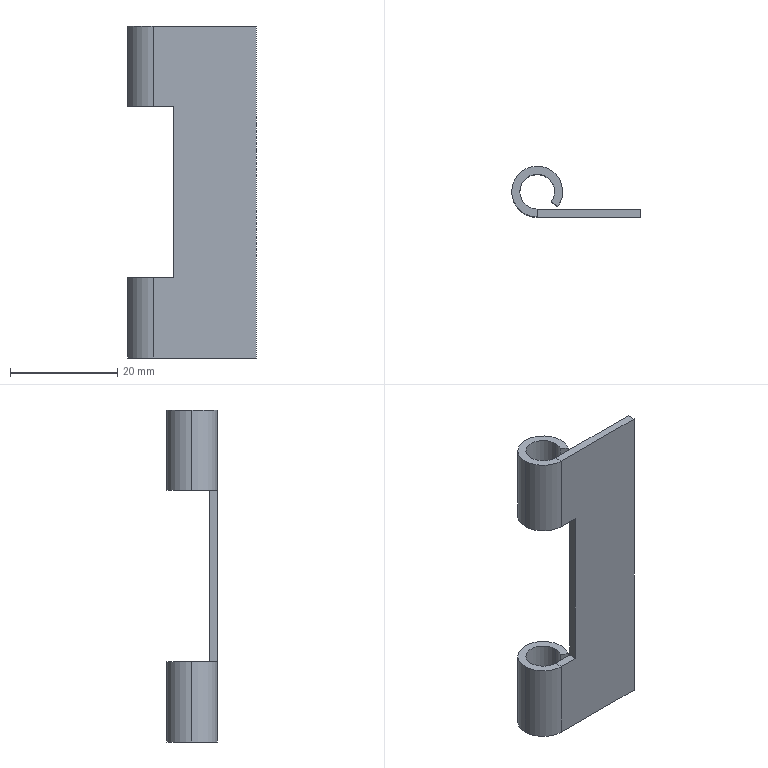Part | SolidWorks | features FlatPattern 1, ICE 1, SMBaseFlange 1, SheetMetal 1 | 1 solid | 26 faces | box 24 x 9.5 x 62 mm | volume 2570 mm3 | plane 14 | cylinder 12 | commonest cylinder face diameters 6.5 x6 9.5 x6
STEP:
#1=CARTESIAN_POINT('',(-24.,4.75,15.));
#2=VERTEX_POINT('',#1);
#3=CARTESIAN_POINT('',(-14.5,4.75,15.));
#4=VERTEX_POINT('',#3);
#5=CARTESIAN_POINT('',(-19.25,4.75,15.));
#6=DIRECTION('',(0.,0.,-1.));
#7=DIRECTION('',(-1.,0.,0.));
#8=AXIS2_PLACEMENT_3D('',#5,#6,#7);
#9=CIRCLE('',#8,4.75);
#10=EDGE_CURVE('',#2,#4,#9,.T.);
#11=ORIENTED_EDGE('',*,*,#10,.T.);
#12=CARTESIAN_POINT('',(-14.5,4.75,0.));
#13=VERTEX_POINT('',#12);
#14=CARTESIAN_POINT('',(-14.5,4.75,62.));
#15=DIRECTION('',(0.,0.,-1.));
#16=VECTOR('',#15,1000.);
#17=LINE('',#14,#16);
#18=EDGE_CURVE('',#4,#13,#17,.T.);
#19=ORIENTED_EDGE('',*,*,#18,.T.);
#20=CARTESIAN_POINT('',(-24.,4.75,0.));
#21=VERTEX_POINT('',#20);
#22=CARTESIAN_POINT('',(-19.25,4.75,0.));
#23=DIRECTION('',(0.,0.,1.));
#24=DIRECTION('',(1.,0.,0.));
#25=AXIS2_PLACEMENT_3D('',#22,#23,#24);
#26=CIRCLE('',#25,4.75);
#27=EDGE_CURVE('',#13,#21,#26,.T.);
#28=ORIENTED_EDGE('',*,*,#27,.T.);
#29=CARTESIAN_POINT('',(-24.,4.75,62.));
#30=DIRECTION('',(0.,0.,-1.));
#31=VECTOR('',#30,1000.);
#32=LINE('',#29,#31);
#33=EDGE_CURVE('',#2,#21,#32,.T.);
#34=ORIENTED_EDGE('',*,*,#33,.F.);
#35=EDGE_LOOP('',(#11,#19,#28,#34));
#36=FACE_OUTER_BOUND('',#35,.T.);
#37=CARTESIAN_POINT('',(-19.25,4.75,62.));
#38=DIRECTION('',(0.,0.,-1.));
#39=DIRECTION('',(-1.,0.,0.));
#40=AXIS2_PLACEMENT_3D('',#37,#38,#39);
#41=CYLINDRICAL_SURFACE('',#40,4.75);
#42=ADVANCED_FACE('',(#36),#41,.T.);
#43=CARTESIAN_POINT('',(-19.25,0.,15.));
#44=VERTEX_POINT('',#43);
#45=CARTESIAN_POINT('',(-19.25,4.75,15.));
#46=DIRECTION('',(0.,0.,-1.));
#47=DIRECTION('',(-1.,0.,0.));
#48=AXIS2_PLACEMENT_3D('',#45,#46,#47);
#49=CIRCLE('',#48,4.75);
#50=EDGE_CURVE('',#44,#2,#49,.T.);
#51=ORIENTED_EDGE('',*,*,#50,.T.);
#52=ORIENTED_EDGE('',*,*,#33,.T.);
#53=CARTESIAN_POINT('',(-19.25,0.,0.));
#54=VERTEX_POINT('',#53);
#55=CARTESIAN_POINT('',(-19.25,4.75,0.));
#56=DIRECTION('',(0.,0.,1.));
#57=DIRECTION('',(1.,0.,0.));
#58=AXIS2_PLACEMENT_3D('',#55,#56,#57);
#59=CIRCLE('',#58,4.75);
#60=EDGE_CURVE('',#21,#54,#59,.T.);
#61=ORIENTED_EDGE('',*,*,#60,.T.);
#62=CARTESIAN_POINT('',(-19.25,0.,62.));
#63=DIRECTION('',(0.,0.,-1.));
#64=VECTOR('',#63,1000.);
#65=LINE('',#62,#64);
#66=EDGE_CURVE('',#44,#54,#65,.T.);
#67=ORIENTED_EDGE('',*,*,#66,.F.);
#68=EDGE_LOOP('',(#51,#52,#61,#67));
#69=FACE_OUTER_BOUND('',#68,.T.);
#70=CARTESIAN_POINT('',(-19.25,4.75,62.));
#71=DIRECTION('',(0.,0.,-1.));
#72=DIRECTION('',(-1.,0.,0.));
#73=AXIS2_PLACEMENT_3D('',#70,#71,#72);
#74=CYLINDRICAL_SURFACE('',#73,4.75);
#75=ADVANCED_FACE('',(#69),#74,.T.);
#76=CARTESIAN_POINT('',(-14.5,4.75,62.));
#77=VERTEX_POINT('',#76);
#78=CARTESIAN_POINT('',(-24.,4.75,62.));
#79=VERTEX_POINT('',#78);
#80=CARTESIAN_POINT('',(-19.25,4.75,62.));
#81=DIRECTION('',(0.,0.,1.));
#82=DIRECTION('',(1.,0.,0.));
#83=AXIS2_PLACEMENT_3D('',#80,#81,#82);
#84=CIRCLE('',#83,4.75);
#85=EDGE_CURVE('',#77,#79,#84,.T.);
#86=ORIENTED_EDGE('',*,*,#85,.F.);
#87=CARTESIAN_POINT('',(-14.5,4.75,47.));
#88=VERTEX_POINT('',#87);
#89=CARTESIAN_POINT('',(-14.5,4.75,62.));
#90=DIRECTION('',(0.,0.,-1.));
#91=VECTOR('',#90,1000.);
#92=LINE('',#89,#91);
#93=EDGE_CURVE('',#77,#88,#92,.T.);
#94=ORIENTED_EDGE('',*,*,#93,.T.);
#95=CARTESIAN_POINT('',(-24.,4.75,47.));
#96=VERTEX_POINT('',#95);
#97=CARTESIAN_POINT('',(-19.25,4.75,47.));
#98=DIRECTION('',(0.,0.,1.));
#99=DIRECTION('',(1.,0.,0.));
#100=AXIS2_PLACEMENT_3D('',#97,#98,#99);
#101=CIRCLE('',#100,4.75);
#102=EDGE_CURVE('',#88,#96,#101,.T.);
#103=ORIENTED_EDGE('',*,*,#102,.T.);
#104=CARTESIAN_POINT('',(-24.,4.75,62.));
#105=DIRECTION('',(0.,0.,-1.));
#106=VECTOR('',#105,1000.);
#107=LINE('',#104,#106);
#108=EDGE_CURVE('',#79,#96,#107,.T.);
#109=ORIENTED_EDGE('',*,*,#108,.F.);
#110=EDGE_LOOP('',(#86,#94,#103,#109));
#111=FACE_OUTER_BOUND('',#110,.T.);
#112=CARTESIAN_POINT('',(-19.25,4.75,62.));
#113=DIRECTION('',(0.,0.,-1.));
#114=DIRECTION('',(-1.,0.,0.));
#115=AXIS2_PLACEMENT_3D('',#112,#113,#114);
#116=CYLINDRICAL_SURFACE('',#115,4.75);
#117=ADVANCED_FACE('',(#111),#116,.T.);
#118=CARTESIAN_POINT('',(-19.25,0.,62.));
#119=VERTEX_POINT('',#118);
#120=CARTESIAN_POINT('',(-19.25,4.75,62.));
#121=DIRECTION('',(0.,0.,1.));
#122=DIRECTION('',(1.,0.,0.));
#123=AXIS2_PLACEMENT_3D('',#120,#121,#122);
#124=CIRCLE('',#123,4.75);
#125=EDGE_CURVE('',#79,#119,#124,.T.);
#126=ORIENTED_EDGE('',*,*,#125,.F.);
#127=ORIENTED_EDGE('',*,*,#108,.T.);
#128=CARTESIAN_POINT('',(-19.25,0.,47.));
#129=VERTEX_POINT('',#128);
#130=CARTESIAN_POINT('',(-19.25,4.75,47.));
#131=DIRECTION('',(0.,0.,1.));
#132=DIRECTION('',(1.,0.,0.));
#133=AXIS2_PLACEMENT_3D('',#130,#131,#132);
#134=CIRCLE('',#133,4.75);
#135=EDGE_CURVE('',#96,#129,#134,.T.);
#136=ORIENTED_EDGE('',*,*,#135,.T.);
#137=CARTESIAN_POINT('',(-19.25,0.,62.));
#138=DIRECTION('',(0.,0.,-1.));
#139=VECTOR('',#138,1000.);
#140=LINE('',#137,#139);
#141=EDGE_CURVE('',#119,#129,#140,.T.);
#142=ORIENTED_EDGE('',*,*,#141,.F.);
#143=EDGE_LOOP('',(#126,#127,#136,#142));
#144=FACE_OUTER_BOUND('',#143,.T.);
#145=CARTESIAN_POINT('',(-19.25,4.75,62.));
#146=DIRECTION('',(0.,0.,-1.));
#147=DIRECTION('',(-1.,0.,0.));
#148=AXIS2_PLACEMENT_3D('',#145,#146,#147);
#149=CYLINDRICAL_SURFACE('',#148,4.75);
#150=ADVANCED_FACE('',(#144),#149,.T.);
#151=CARTESIAN_POINT('',(-16.,4.75,15.));
#152=VERTEX_POINT('',#151);
#153=CARTESIAN_POINT('',(-16.6,2.868,15.));
#154=VERTEX_POINT('',#153);
#155=CARTESIAN_POINT('',(-19.25,4.75,15.));
#156=DIRECTION('',(0.,0.,-1.));
#157=DIRECTION('',(-1.,0.,0.));
#158=AXIS2_PLACEMENT_3D('',#155,#156,#157);
#159=CIRCLE('',#158,3.25);
#160=EDGE_CURVE('',#152,#154,#159,.T.);
#161=ORIENTED_EDGE('',*,*,#160,.F.);
#162=CARTESIAN_POINT('',(-16.,4.75,0.));
#163=VERTEX_POINT('',#162);
#164=CARTESIAN_POINT('',(-16.,4.75,62.));
#165=DIRECTION('',(0.,0.,-1.));
#166=VECTOR('',#165,1000.);
#167=LINE('',#164,#166);
#168=EDGE_CURVE('',#152,#163,#167,.T.);
#169=ORIENTED_EDGE('',*,*,#168,.T.);
#170=CARTESIAN_POINT('',(-16.6,2.868,0.));
#171=VERTEX_POINT('',#170);
#172=CARTESIAN_POINT('',(-19.25,4.75,0.));
#173=DIRECTION('',(0.,0.,1.));
#174=DIRECTION('',(1.,0.,0.));
#175=AXIS2_PLACEMENT_3D('',#172,#173,#174);
#176=CIRCLE('',#175,3.25);
#177=EDGE_CURVE('',#171,#163,#176,.T.);
#178=ORIENTED_EDGE('',*,*,#177,.F.);
#179=CARTESIAN_POINT('',(-16.6,2.868,62.));
#180=DIRECTION('',(0.,0.,-1.));
#181=VECTOR('',#180,1000.);
#182=LINE('',#179,#181);
#183=EDGE_CURVE('',#154,#171,#182,.T.);
#184=ORIENTED_EDGE('',*,*,#183,.F.);
#185=EDGE_LOOP('',(#161,#169,#178,#184));
#186=FACE_OUTER_BOUND('',#185,.T.);
#187=CARTESIAN_POINT('',(-19.25,4.75,62.));
#188=DIRECTION('',(0.,0.,-1.));
#189=DIRECTION('',(-1.,0.,0.));
#190=AXIS2_PLACEMENT_3D('',#187,#188,#189);
#191=CYLINDRICAL_SURFACE('',#190,3.25);
#192=ADVANCED_FACE('',(#186),#191,.F.);
#193=ORIENTED_EDGE('',*,*,#168,.F.);
#194=CARTESIAN_POINT('',(-22.5,4.75,15.));
#195=VERTEX_POINT('',#194);
#196=CARTESIAN_POINT('',(-19.25,4.75,15.));
#197=DIRECTION('',(0.,0.,-1.));
#198=DIRECTION('',(-1.,0.,0.));
#199=AXIS2_PLACEMENT_3D('',#196,#197,#198);
#200=CIRCLE('',#199,3.25);
#201=EDGE_CURVE('',#195,#152,#200,.T.);
#202=ORIENTED_EDGE('',*,*,#201,.F.);
#203=CARTESIAN_POINT('',(-22.5,4.75,0.));
#204=VERTEX_POINT('',#203);
#205=CARTESIAN_POINT('',(-22.5,4.75,62.));
#206=DIRECTION('',(0.,0.,-1.));
#207=VECTOR('',#206,1000.);
#208=LINE('',#205,#207);
#209=EDGE_CURVE('',#195,#204,#208,.T.);
#210=ORIENTED_EDGE('',*,*,#209,.T.);
#211=CARTESIAN_POINT('',(-19.25,4.75,0.));
#212=DIRECTION('',(0.,0.,1.));
#213=DIRECTION('',(1.,0.,0.));
#214=AXIS2_PLACEMENT_3D('',#211,#212,#213);
#215=CIRCLE('',#214,3.25);
#216=EDGE_CURVE('',#163,#204,#215,.T.);
#217=ORIENTED_EDGE('',*,*,#216,.F.);
#218=EDGE_LOOP('',(#193,#202,#210,#217));
#219=FACE_OUTER_BOUND('',#218,.T.);
#220=CARTESIAN_POINT('',(-19.25,4.75,62.));
#221=DIRECTION('',(0.,0.,-1.));
#222=DIRECTION('',(-1.,0.,0.));
#223=AXIS2_PLACEMENT_3D('',#220,#221,#222);
#224=CYLINDRICAL_SURFACE('',#223,3.25);
#225=ADVANCED_FACE('',(#219),#224,.F.);
#226=CARTESIAN_POINT('',(-16.6,2.868,62.));
#227=VERTEX_POINT('',#226);
#228=CARTESIAN_POINT('',(-16.,4.75,62.));
#229=VERTEX_POINT('',#228);
#230=CARTESIAN_POINT('',(-19.25,4.75,62.));
#231=DIRECTION('',(0.,0.,1.));
#232=DIRECTION('',(1.,0.,0.));
#233=AXIS2_PLACEMENT_3D('',#230,#231,#232);
#234=CIRCLE('',#233,3.25);
#235=EDGE_CURVE('',#227,#229,#234,.T.);
#236=ORIENTED_EDGE('',*,*,#235,.T.);
#237=CARTESIAN_POINT('',(-16.,4.75,47.));
#238=VERTEX_POINT('',#237);
#239=CARTESIAN_POINT('',(-16.,4.75,62.));
#240=DIRECTION('',(0.,0.,-1.));
#241=VECTOR('',#240,1000.);
#242=LINE('',#239,#241);
#243=EDGE_CURVE('',#229,#238,#242,.T.);
#244=ORIENTED_EDGE('',*,*,#243,.T.);
#245=CARTESIAN_POINT('',(-16.6,2.868,47.));
#246=VERTEX_POINT('',#245);
#247=CARTESIAN_POINT('',(-19.25,4.75,47.));
#248=DIRECTION('',(0.,0.,1.));
#249=DIRECTION('',(-1.,0.,0.));
#250=AXIS2_PLACEMENT_3D('',#247,#248,#249);
#251=CIRCLE('',#250,3.25);
#252=EDGE_CURVE('',#246,#238,#251,.T.);
#253=ORIENTED_EDGE('',*,*,#252,.F.);
#254=CARTESIAN_POINT('',(-16.6,2.868,62.));
#255=DIRECTION('',(0.,0.,-1.));
#256=VECTOR('',#255,1000.);
#257=LINE('',#254,#256);
#258=EDGE_CURVE('',#227,#246,#257,.T.);
#259=ORIENTED_EDGE('',*,*,#258,.F.);
#260=EDGE_LOOP('',(#236,#244,#253,#259));
#261=FACE_OUTER_BOUND('',#260,.T.);
#262=CARTESIAN_POINT('',(-19.25,4.75,62.));
#263=DIRECTION('',(0.,0.,-1.));
#264=DIRECTION('',(-1.,0.,0.));
#265=AXIS2_PLACEMENT_3D('',#262,#263,#264);
#266=CYLINDRICAL_SURFACE('',#265,3.25);
#267=ADVANCED_FACE('',(#261),#266,.F.);
#268=ORIENTED_EDGE('',*,*,#243,.F.);
#269=CARTESIAN_POINT('',(-22.5,4.75,62.));
#270=VERTEX_POINT('',#269);
#271=CARTESIAN_POINT('',(-19.25,4.75,62.));
#272=DIRECTION('',(0.,0.,1.));
#273=DIRECTION('',(1.,0.,0.));
#274=AXIS2_PLACEMENT_3D('',#271,#272,#273);
#275=CIRCLE('',#274,3.25);
#276=EDGE_CURVE('',#229,#270,#275,.T.);
#277=ORIENTED_EDGE('',*,*,#276,.T.);
#278=CARTESIAN_POINT('',(-22.5,4.75,47.));
#279=VERTEX_POINT('',#278);
#280=CARTESIAN_POINT('',(-22.5,4.75,62.));
#281=DIRECTION('',(0.,0.,-1.));
#282=VECTOR('',#281,1000.);
#283=LINE('',#280,#282);
#284=EDGE_CURVE('',#270,#279,#283,.T.);
#285=ORIENTED_EDGE('',*,*,#284,.T.);
#286=CARTESIAN_POINT('',(-19.25,4.75,47.));
#287=DIRECTION('',(0.,0.,1.));
#288=DIRECTION('',(-1.,0.,0.));
#289=AXIS2_PLACEMENT_3D('',#286,#287,#288);
#290=CIRCLE('',#289,3.25);
#291=EDGE_CURVE('',#238,#279,#290,.T.);
#292=ORIENTED_EDGE('',*,*,#291,.F.);
#293=EDGE_LOOP('',(#268,#277,#285,#292));
#294=FACE_OUTER_BOUND('',#293,.T.);
#295=CARTESIAN_POINT('',(-19.25,4.75,62.));
#296=DIRECTION('',(0.,0.,-1.));
#297=DIRECTION('',(-1.,0.,0.));
#298=AXIS2_PLACEMENT_3D('',#295,#296,#297);
#299=CYLINDRICAL_SURFACE('',#298,3.25);
#300=ADVANCED_FACE('',(#294),#299,.F.);
#301=CARTESIAN_POINT('',(-15.5,0.,47.));
#302=VERTEX_POINT('',#301);
#303=CARTESIAN_POINT('',(0.,0.,47.));
#304=DIRECTION('',(1.,0.,0.));
#305=VECTOR('',#304,1000.);
#306=LINE('',#303,#305);
#307=EDGE_CURVE('',#129,#302,#306,.T.);
#308=ORIENTED_EDGE('',*,*,#307,.T.);
#309=CARTESIAN_POINT('',(-15.5,0.,15.));
#310=VERTEX_POINT('',#309);
#311=CARTESIAN_POINT('',(-15.5,0.,62.));
#312=DIRECTION('',(0.,0.,-1.));
#313=VECTOR('',#312,1000.);
#314=LINE('',#311,#313);
#315=EDGE_CURVE('',#302,#310,#314,.T.);
#316=ORIENTED_EDGE('',*,*,#315,.T.);
#317=CARTESIAN_POINT('',(0.,0.,15.));
#318=DIRECTION('',(-1.,0.,0.));
#319=VECTOR('',#318,1000.);
#320=LINE('',#317,#319);
#321=EDGE_CURVE('',#310,#44,#320,.T.);
#322=ORIENTED_EDGE('',*,*,#321,.T.);
#323=ORIENTED_EDGE('',*,*,#66,.T.);
#324=CARTESIAN_POINT('',(0.,0.,0.));
#325=VERTEX_POINT('',#324);
#326=CARTESIAN_POINT('',(0.,0.,0.));
#327=DIRECTION('',(1.,0.,0.));
#328=VECTOR('',#327,1000.);
#329=LINE('',#326,#328);
#330=EDGE_CURVE('',#54,#325,#329,.T.);
#331=ORIENTED_EDGE('',*,*,#330,.T.);
#332=CARTESIAN_POINT('',(0.,0.,62.));
#333=VERTEX_POINT('',#332);
#334=CARTESIAN_POINT('',(0.,0.,62.));
#335=DIRECTION('',(0.,0.,-1.));
#336=VECTOR('',#335,1000.);
#337=LINE('',#334,#336);
#338=EDGE_CURVE('',#333,#325,#337,.T.);
#339=ORIENTED_EDGE('',*,*,#338,.F.);
#340=CARTESIAN_POINT('',(0.,0.,62.));
#341=DIRECTION('',(1.,0.,0.));
#342=VECTOR('',#341,1000.);
#343=LINE('',#340,#342);
#344=EDGE_CURVE('',#119,#333,#343,.T.);
#345=ORIENTED_EDGE('',*,*,#344,.F.);
#346=ORIENTED_EDGE('',*,*,#141,.T.);
#347=EDGE_LOOP('',(#308,#316,#322,#323,#331,#339,#345,#346));
#348=FACE_OUTER_BOUND('',#347,.T.);
#349=CARTESIAN_POINT('',(0.,0.,62.));
#350=DIRECTION('',(0.,1.,0.));
#351=DIRECTION('',(-1.,0.,0.));
#352=AXIS2_PLACEMENT_3D('',#349,#350,#351);
#353=PLANE('',#352);
#354=ADVANCED_FACE('',(#348),#353,.F.);
#355=CARTESIAN_POINT('',(-15.5,1.5,47.));
#356=VERTEX_POINT('',#355);
#357=CARTESIAN_POINT('',(-15.5,1.5,15.));
#358=VERTEX_POINT('',#357);
#359=CARTESIAN_POINT('',(-15.5,1.5,62.));
#360=DIRECTION('',(0.,0.,-1.));
#361=VECTOR('',#360,1000.);
#362=LINE('',#359,#361);
#363=EDGE_CURVE('',#356,#358,#362,.T.);
#364=ORIENTED_EDGE('',*,*,#363,.F.);
#365=CARTESIAN_POINT('',(-19.25,1.5,47.));
#366=VERTEX_POINT('',#365);
#367=CARTESIAN_POINT('',(0.,1.5,47.));
#368=DIRECTION('',(1.,0.,0.));
#369=VECTOR('',#368,1000.);
#370=LINE('',#367,#369);
#371=EDGE_CURVE('',#366,#356,#370,.T.);
#372=ORIENTED_EDGE('',*,*,#371,.F.);
#373=CARTESIAN_POINT('',(-19.25,1.5,62.));
#374=VERTEX_POINT('',#373);
#375=CARTESIAN_POINT('',(-19.25,1.5,62.));
#376=DIRECTION('',(0.,0.,-1.));
#377=VECTOR('',#376,1000.);
#378=LINE('',#375,#377);
#379=EDGE_CURVE('',#374,#366,#378,.T.);
#380=ORIENTED_EDGE('',*,*,#379,.F.);
#381=CARTESIAN_POINT('',(0.,1.5,62.));
#382=VERTEX_POINT('',#381);
#383=CARTESIAN_POINT('',(0.,1.5,62.));
#384=DIRECTION('',(1.,0.,0.));
#385=VECTOR('',#384,1000.);
#386=LINE('',#383,#385);
#387=EDGE_CURVE('',#374,#382,#386,.T.);
#388=ORIENTED_EDGE('',*,*,#387,.T.);
#389=CARTESIAN_POINT('',(0.,1.5,0.));
#390=VERTEX_POINT('',#389);
#391=CARTESIAN_POINT('',(0.,1.5,62.));
#392=DIRECTION('',(0.,0.,-1.));
#393=VECTOR('',#392,1000.);
#394=LINE('',#391,#393);
#395=EDGE_CURVE('',#382,#390,#394,.T.);
#396=ORIENTED_EDGE('',*,*,#395,.T.);
#397=CARTESIAN_POINT('',(-19.25,1.5,0.));
#398=VERTEX_POINT('',#397);
#399=CARTESIAN_POINT('',(0.,1.5,0.));
#400=DIRECTION('',(1.,0.,0.));
#401=VECTOR('',#400,1000.);
#402=LINE('',#399,#401);
#403=EDGE_CURVE('',#398,#390,#402,.T.);
#404=ORIENTED_EDGE('',*,*,#403,.F.);
#405=CARTESIAN_POINT('',(-19.25,1.5,15.));
#406=VERTEX_POINT('',#405);
#407=CARTESIAN_POINT('',(-19.25,1.5,62.));
#408=DIRECTION('',(0.,0.,-1.));
#409=VECTOR('',#408,1000.);
#410=LINE('',#407,#409);
#411=EDGE_CURVE('',#406,#398,#410,.T.);
#412=ORIENTED_EDGE('',*,*,#411,.F.);
#413=CARTESIAN_POINT('',(0.,1.5,15.));
#414=DIRECTION('',(-1.,0.,0.));
#415=VECTOR('',#414,1000.);
#416=LINE('',#413,#415);
#417=EDGE_CURVE('',#358,#406,#416,.T.);
#418=ORIENTED_EDGE('',*,*,#417,.F.);
#419=EDGE_LOOP('',(#364,#372,#380,#388,#396,#404,#412,#418));
#420=FACE_OUTER_BOUND('',#419,.T.);
#421=CARTESIAN_POINT('',(0.,1.5,62.));
#422=DIRECTION('',(0.,1.,0.));
#423=DIRECTION('',(-1.,0.,0.));
#424=AXIS2_PLACEMENT_3D('',#421,#422,#423);
#425=PLANE('',#424);
#426=ADVANCED_FACE('',(#420),#425,.T.);
#427=ORIENTED_EDGE('',*,*,#284,.F.);
#428=CARTESIAN_POINT('',(-19.25,4.75,62.));
#429=DIRECTION('',(0.,0.,1.));
#430=DIRECTION('',(1.,0.,0.));
#431=AXIS2_PLACEMENT_3D('',#428,#429,#430);
#432=CIRCLE('',#431,3.25);
#433=EDGE_CURVE('',#270,#374,#432,.T.);
#434=ORIENTED_EDGE('',*,*,#433,.T.);
#435=ORIENTED_EDGE('',*,*,#379,.T.);
#436=CARTESIAN_POINT('',(-19.25,4.75,47.));
#437=DIRECTION('',(0.,0.,1.));
#438=DIRECTION('',(-1.,0.,0.));
#439=AXIS2_PLACEMENT_3D('',#436,#437,#438);
#440=CIRCLE('',#439,3.25);
#441=EDGE_CURVE('',#279,#366,#440,.T.);
#442=ORIENTED_EDGE('',*,*,#441,.F.);
#443=EDGE_LOOP('',(#427,#434,#435,#442));
#444=FACE_OUTER_BOUND('',#443,.T.);
#445=CARTESIAN_POINT('',(-19.25,4.75,62.));
#446=DIRECTION('',(0.,0.,-1.));
#447=DIRECTION('',(-1.,0.,0.));
#448=AXIS2_PLACEMENT_3D('',#445,#446,#447);
#449=CYLINDRICAL_SURFACE('',#448,3.25);
#450=ADVANCED_FACE('',(#444),#449,.F.);
#451=ORIENTED_EDGE('',*,*,#209,.F.);
#452=CARTESIAN_POINT('',(-19.25,4.75,15.));
#453=DIRECTION('',(0.,0.,-1.));
#454=DIRECTION('',(-1.,0.,0.));
#455=AXIS2_PLACEMENT_3D('',#452,#453,#454);
#456=CIRCLE('',#455,3.25);
#457=EDGE_CURVE('',#406,#195,#456,.T.);
#458=ORIENTED_EDGE('',*,*,#457,.F.);
#459=ORIENTED_EDGE('',*,*,#411,.T.);
#460=CARTESIAN_POINT('',(-19.25,4.75,0.));
#461=DIRECTION('',(0.,0.,1.));
#462=DIRECTION('',(1.,0.,0.));
#463=AXIS2_PLACEMENT_3D('',#460,#461,#462);
#464=CIRCLE('',#463,3.25);
#465=EDGE_CURVE('',#204,#398,#464,.T.);
#466=ORIENTED_EDGE('',*,*,#465,.F.);
#467=EDGE_LOOP('',(#451,#458,#459,#466));
#468=FACE_OUTER_BOUND('',#467,.T.);
#469=CARTESIAN_POINT('',(-19.25,4.75,62.));
#470=DIRECTION('',(0.,0.,-1.));
#471=DIRECTION('',(-1.,0.,0.));
#472=AXIS2_PLACEMENT_3D('',#469,#470,#471);
#473=CYLINDRICAL_SURFACE('',#472,3.25);
#474=ADVANCED_FACE('',(#468),#473,.F.);
#475=ORIENTED_EDGE('',*,*,#258,.T.);
#476=CARTESIAN_POINT('',(-15.377,2.,47.));
#477=VERTEX_POINT('',#476);
#478=CARTESIAN_POINT('',(-16.6,2.868,47.));
#479=DIRECTION('',(0.8154,-0.5789,0.));
#480=VECTOR('',#479,1000.);
#481=LINE('',#478,#480);
#482=EDGE_CURVE('',#246,#477,#481,.T.);
#483=ORIENTED_EDGE('',*,*,#482,.T.);
#484=CARTESIAN_POINT('',(-15.377,2.,62.));
#485=VERTEX_POINT('',#484);
#486=CARTESIAN_POINT('',(-15.377,2.,62.));
#487=DIRECTION('',(0.,0.,-1.));
#488=VECTOR('',#487,1000.);
#489=LINE('',#486,#488);
#490=EDGE_CURVE('',#485,#477,#489,.T.);
#491=ORIENTED_EDGE('',*,*,#490,.F.);
#492=CARTESIAN_POINT('',(-15.377,2.,62.));
#493=DIRECTION('',(-0.8154,0.5789,0.));
#494=VECTOR('',#493,1000.);
#495=LINE('',#492,#494);
#496=EDGE_CURVE('',#485,#227,#495,.T.);
#497=ORIENTED_EDGE('',*,*,#496,.T.);
#498=EDGE_LOOP('',(#475,#483,#491,#497));
#499=FACE_OUTER_BOUND('',#498,.T.);
#500=CARTESIAN_POINT('',(-15.377,2.,62.));
#501=DIRECTION('',(-0.5789,-0.8154,0.));
#502=DIRECTION('',(0.8154,-0.5789,0.));
#503=AXIS2_PLACEMENT_3D('',#500,#501,#502);
#504=PLANE('',#503);
#505=ADVANCED_FACE('',(#499),#504,.T.);
#506=CARTESIAN_POINT('',(-15.377,2.,15.));
#507=VERTEX_POINT('',#506);
#508=CARTESIAN_POINT('',(-15.377,2.,0.));
#509=VERTEX_POINT('',#508);
#510=CARTESIAN_POINT('',(-15.377,2.,62.));
#511=DIRECTION('',(0.,0.,-1.));
#512=VECTOR('',#511,1000.);
#513=LINE('',#510,#512);
#514=EDGE_CURVE('',#507,#509,#513,.T.);
#515=ORIENTED_EDGE('',*,*,#514,.F.);
#516=CARTESIAN_POINT('',(-16.6,2.868,15.));
#517=DIRECTION('',(0.8154,-0.5789,0.));
#518=VECTOR('',#517,1000.);
#519=LINE('',#516,#518);
#520=EDGE_CURVE('',#154,#507,#519,.T.);
#521=ORIENTED_EDGE('',*,*,#520,.F.);
#522=ORIENTED_EDGE('',*,*,#183,.T.);
#523=CARTESIAN_POINT('',(-15.377,2.,0.));
#524=DIRECTION('',(-0.8154,0.5789,0.));
#525=VECTOR('',#524,1000.);
#526=LINE('',#523,#525);
#527=EDGE_CURVE('',#509,#171,#526,.T.);
#528=ORIENTED_EDGE('',*,*,#527,.F.);
#529=EDGE_LOOP('',(#515,#521,#522,#528));
#530=FACE_OUTER_BOUND('',#529,.T.);
#531=CARTESIAN_POINT('',(-15.377,2.,62.));
#532=DIRECTION('',(-0.5789,-0.8154,0.));
#533=DIRECTION('',(0.8154,-0.5789,0.));
#534=AXIS2_PLACEMENT_3D('',#531,#532,#533);
#535=PLANE('',#534);
#536=ADVANCED_FACE('',(#530),#535,.T.);
#537=ORIENTED_EDGE('',*,*,#93,.F.);
#538=CARTESIAN_POINT('',(-19.25,4.75,62.));
#539=DIRECTION('',(0.,0.,1.));
#540=DIRECTION('',(1.,0.,0.));
#541=AXIS2_PLACEMENT_3D('',#538,#539,#540);
#542=CIRCLE('',#541,4.75);
#543=EDGE_CURVE('',#485,#77,#542,.T.);
#544=ORIENTED_EDGE('',*,*,#543,.F.);
#545=ORIENTED_EDGE('',*,*,#490,.T.);
#546=CARTESIAN_POINT('',(-19.25,4.75,47.));
#547=DIRECTION('',(0.,0.,1.));
#548=DIRECTION('',(1.,0.,0.));
#549=AXIS2_PLACEMENT_3D('',#546,#547,#548);
#550=CIRCLE('',#549,4.75);
#551=EDGE_CURVE('',#477,#88,#550,.T.);
#552=ORIENTED_EDGE('',*,*,#551,.T.);
#553=EDGE_LOOP('',(#537,#544,#545,#552));
#554=FACE_OUTER_BOUND('',#553,.T.);
#555=CARTESIAN_POINT('',(-19.25,4.75,62.));
#556=DIRECTION('',(0.,0.,-1.));
#557=DIRECTION('',(-1.,0.,0.));
#558=AXIS2_PLACEMENT_3D('',#555,#556,#557);
#559=CYLINDRICAL_SURFACE('',#558,4.75);
#560=ADVANCED_FACE('',(#554),#559,.T.);
#561=ORIENTED_EDGE('',*,*,#18,.F.);
#562=CARTESIAN_POINT('',(-19.25,4.75,15.));
#563=DIRECTION('',(0.,0.,-1.));
#564=DIRECTION('',(-1.,0.,0.));
#565=AXIS2_PLACEMENT_3D('',#562,#563,#564);
#566=CIRCLE('',#565,4.75);
#567=EDGE_CURVE('',#4,#507,#566,.T.);
#568=ORIENTED_EDGE('',*,*,#567,.T.);
#569=ORIENTED_EDGE('',*,*,#514,.T.);
#570=CARTESIAN_POINT('',(-19.25,4.75,0.));
#571=DIRECTION('',(0.,0.,1.));
#572=DIRECTION('',(1.,0.,0.));
#573=AXIS2_PLACEMENT_3D('',#570,#571,#572);
#574=CIRCLE('',#573,4.75);
#575=EDGE_CURVE('',#509,#13,#574,.T.);
#576=ORIENTED_EDGE('',*,*,#575,.T.);
#577=EDGE_LOOP('',(#561,#568,#569,#576));
#578=FACE_OUTER_BOUND('',#577,.T.);
#579=CARTESIAN_POINT('',(-19.25,4.75,62.));
#580=DIRECTION('',(0.,0.,-1.));
#581=DIRECTION('',(-1.,0.,0.));
#582=AXIS2_PLACEMENT_3D('',#579,#580,#581);
#583=CYLINDRICAL_SURFACE('',#582,4.75);
#584=ADVANCED_FACE('',(#578),#583,.T.);
#585=CARTESIAN_POINT('',(-19.25,1.5,62.));
#586=DIRECTION('',(0.,-1.,0.));
#587=VECTOR('',#586,1000.);
#588=LINE('',#585,#587);
#589=EDGE_CURVE('',#374,#119,#588,.T.);
#590=ORIENTED_EDGE('',*,*,#589,.F.);
#591=ORIENTED_EDGE('',*,*,#433,.F.);
#592=ORIENTED_EDGE('',*,*,#276,.F.);
#593=ORIENTED_EDGE('',*,*,#235,.F.);
#594=ORIENTED_EDGE('',*,*,#496,.F.);
#595=ORIENTED_EDGE('',*,*,#543,.T.);
#596=ORIENTED_EDGE('',*,*,#85,.T.);
#597=ORIENTED_EDGE('',*,*,#125,.T.);
#598=EDGE_LOOP('',(#590,#591,#592,#593,#594,#595,#596,#597));
#599=FACE_OUTER_BOUND('',#598,.T.);
#600=CARTESIAN_POINT('',(-19.25,1.5,62.));
#601=DIRECTION('',(0.,0.,1.));
#602=DIRECTION('',(1.,0.,0.));
#603=AXIS2_PLACEMENT_3D('',#600,#601,#602);
#604=PLANE('',#603);
#605=ADVANCED_FACE('',(#599),#604,.T.);
#606=CARTESIAN_POINT('',(-19.25,0.,0.));
#607=DIRECTION('',(0.,1.,0.));
#608=VECTOR('',#607,1000.);
#609=LINE('',#606,#608);
#610=EDGE_CURVE('',#54,#398,#609,.T.);
#611=ORIENTED_EDGE('',*,*,#610,.F.);
#612=ORIENTED_EDGE('',*,*,#60,.F.);
#613=ORIENTED_EDGE('',*,*,#27,.F.);
#614=ORIENTED_EDGE('',*,*,#575,.F.);
#615=ORIENTED_EDGE('',*,*,#527,.T.);
#616=ORIENTED_EDGE('',*,*,#177,.T.);
#617=ORIENTED_EDGE('',*,*,#216,.T.);
#618=ORIENTED_EDGE('',*,*,#465,.T.);
#619=EDGE_LOOP('',(#611,#612,#613,#614,#615,#616,#617,#618));
#620=FACE_OUTER_BOUND('',#619,.T.);
#621=CARTESIAN_POINT('',(-19.25,0.,0.));
#622=DIRECTION('',(0.,0.,-1.));
#623=DIRECTION('',(-1.,0.,0.));
#624=AXIS2_PLACEMENT_3D('',#621,#622,#623);
#625=PLANE('',#624);
#626=ADVANCED_FACE('',(#620),#625,.T.);
#627=CARTESIAN_POINT('',(0.,1.5,0.));
#628=DIRECTION('',(0.,-1.,0.));
#629=VECTOR('',#628,1000.);
#630=LINE('',#627,#629);
#631=EDGE_CURVE('',#390,#325,#630,.T.);
#632=ORIENTED_EDGE('',*,*,#631,.F.);
#633=ORIENTED_EDGE('',*,*,#395,.F.);
#634=CARTESIAN_POINT('',(0.,1.5,62.));
#635=DIRECTION('',(0.,-1.,0.));
#636=VECTOR('',#635,1000.);
#637=LINE('',#634,#636);
#638=EDGE_CURVE('',#382,#333,#637,.T.);
#639=ORIENTED_EDGE('',*,*,#638,.T.);
#640=ORIENTED_EDGE('',*,*,#338,.T.);
#641=EDGE_LOOP('',(#632,#633,#639,#640));
#642=FACE_OUTER_BOUND('',#641,.T.);
#643=CARTESIAN_POINT('',(0.,1.5,62.));
#644=DIRECTION('',(1.,0.,0.));
#645=DIRECTION('',(0.,1.,0.));
#646=AXIS2_PLACEMENT_3D('',#643,#644,#645);
#647=PLANE('',#646);
#648=ADVANCED_FACE('',(#642),#647,.T.);
#649=ORIENTED_EDGE('',*,*,#344,.T.);
#650=ORIENTED_EDGE('',*,*,#638,.F.);
#651=ORIENTED_EDGE('',*,*,#387,.F.);
#652=ORIENTED_EDGE('',*,*,#589,.T.);
#653=EDGE_LOOP('',(#649,#650,#651,#652));
#654=FACE_OUTER_BOUND('',#653,.T.);
#655=CARTESIAN_POINT('',(-19.25,4.75,62.));
#656=DIRECTION('',(0.,0.,1.));
#657=DIRECTION('',(1.,0.,0.));
#658=AXIS2_PLACEMENT_3D('',#655,#656,#657);
#659=PLANE('',#658);
#660=ADVANCED_FACE('',(#654),#659,.T.);
#661=ORIENTED_EDGE('',*,*,#330,.F.);
#662=ORIENTED_EDGE('',*,*,#610,.T.);
#663=ORIENTED_EDGE('',*,*,#403,.T.);
#664=ORIENTED_EDGE('',*,*,#631,.T.);
#665=EDGE_LOOP('',(#661,#662,#663,#664));
#666=FACE_OUTER_BOUND('',#665,.T.);
#667=CARTESIAN_POINT('',(-19.25,4.75,0.));
#668=DIRECTION('',(0.,0.,1.));
#669=DIRECTION('',(1.,0.,0.));
#670=AXIS2_PLACEMENT_3D('',#667,#668,#669);
#671=PLANE('',#670);
#672=ADVANCED_FACE('',(#666),#671,.F.);
#673=CARTESIAN_POINT('',(-19.25,1.5,47.));
#674=DIRECTION('',(0.,-1.,0.));
#675=VECTOR('',#674,1000.);
#676=LINE('',#673,#675);
#677=EDGE_CURVE('',#366,#129,#676,.T.);
#678=ORIENTED_EDGE('',*,*,#677,.F.);
#679=ORIENTED_EDGE('',*,*,#371,.T.);
#680=CARTESIAN_POINT('',(-15.5,1.5,47.));
#681=DIRECTION('',(0.,-1.,0.));
#682=VECTOR('',#681,1000.);
#683=LINE('',#680,#682);
#684=EDGE_CURVE('',#356,#302,#683,.T.);
#685=ORIENTED_EDGE('',*,*,#684,.T.);
#686=ORIENTED_EDGE('',*,*,#307,.F.);
#687=EDGE_LOOP('',(#678,#679,#685,#686));
#688=FACE_OUTER_BOUND('',#687,.T.);
#689=CARTESIAN_POINT('',(0.,1.5,47.));
#690=DIRECTION('',(0.,0.,1.));
#691=DIRECTION('',(1.,0.,0.));
#692=AXIS2_PLACEMENT_3D('',#689,#690,#691);
#693=PLANE('',#692);
#694=ADVANCED_FACE('',(#688),#693,.F.);
#695=ORIENTED_EDGE('',*,*,#684,.F.);
#696=ORIENTED_EDGE('',*,*,#363,.T.);
#697=CARTESIAN_POINT('',(-15.5,1.5,15.));
#698=DIRECTION('',(0.,-1.,0.));
#699=VECTOR('',#698,1000.);
#700=LINE('',#697,#699);
#701=EDGE_CURVE('',#358,#310,#700,.T.);
#702=ORIENTED_EDGE('',*,*,#701,.T.);
#703=ORIENTED_EDGE('',*,*,#315,.F.);
#704=EDGE_LOOP('',(#695,#696,#702,#703));
#705=FACE_OUTER_BOUND('',#704,.T.);
#706=CARTESIAN_POINT('',(-15.5,1.5,62.));
#707=DIRECTION('',(1.,0.,0.));
#708=DIRECTION('',(0.,0.,-1.));
#709=AXIS2_PLACEMENT_3D('',#706,#707,#708);
#710=PLANE('',#709);
#711=ADVANCED_FACE('',(#705),#710,.F.);
#712=ORIENTED_EDGE('',*,*,#417,.T.);
#713=CARTESIAN_POINT('',(-19.25,1.5,15.));
#714=DIRECTION('',(0.,-1.,0.));
#715=VECTOR('',#714,1000.);
#716=LINE('',#713,#715);
#717=EDGE_CURVE('',#406,#44,#716,.T.);
#718=ORIENTED_EDGE('',*,*,#717,.T.);
#719=ORIENTED_EDGE('',*,*,#321,.F.);
#720=ORIENTED_EDGE('',*,*,#701,.F.);
#721=EDGE_LOOP('',(#712,#718,#719,#720));
#722=FACE_OUTER_BOUND('',#721,.T.);
#723=CARTESIAN_POINT('',(0.,1.5,15.));
#724=DIRECTION('',(0.,0.,-1.));
#725=DIRECTION('',(-1.,0.,0.));
#726=AXIS2_PLACEMENT_3D('',#723,#724,#725);
#727=PLANE('',#726);
#728=ADVANCED_FACE('',(#722),#727,.F.);
#729=ORIENTED_EDGE('',*,*,#677,.T.);
#730=ORIENTED_EDGE('',*,*,#135,.F.);
#731=ORIENTED_EDGE('',*,*,#102,.F.);
#732=ORIENTED_EDGE('',*,*,#551,.F.);
#733=ORIENTED_EDGE('',*,*,#482,.F.);
#734=ORIENTED_EDGE('',*,*,#252,.T.);
#735=ORIENTED_EDGE('',*,*,#291,.T.);
#736=ORIENTED_EDGE('',*,*,#441,.T.);
#737=EDGE_LOOP('',(#729,#730,#731,#732,#733,#734,#735,#736));
#738=FACE_OUTER_BOUND('',#737,.T.);
#739=CARTESIAN_POINT('',(-19.25,4.75,47.));
#740=DIRECTION('',(0.,0.,-1.));
#741=DIRECTION('',(-1.,0.,0.));
#742=AXIS2_PLACEMENT_3D('',#739,#740,#741);
#743=PLANE('',#742);
#744=ADVANCED_FACE('',(#738),#743,.T.);
#745=ORIENTED_EDGE('',*,*,#457,.T.);
#746=ORIENTED_EDGE('',*,*,#201,.T.);
#747=ORIENTED_EDGE('',*,*,#160,.T.);
#748=ORIENTED_EDGE('',*,*,#520,.T.);
#749=ORIENTED_EDGE('',*,*,#567,.F.);
#750=ORIENTED_EDGE('',*,*,#10,.F.);
#751=ORIENTED_EDGE('',*,*,#50,.F.);
#752=ORIENTED_EDGE('',*,*,#717,.F.);
#753=EDGE_LOOP('',(#745,#746,#747,#748,#749,#750,#751,#752));
#754=FACE_OUTER_BOUND('',#753,.T.);
#755=CARTESIAN_POINT('',(-19.25,4.75,15.));
#756=DIRECTION('',(0.,0.,1.));
#757=DIRECTION('',(1.,0.,0.));
#758=AXIS2_PLACEMENT_3D('',#755,#756,#757);
#759=PLANE('',#758);
#760=ADVANCED_FACE('',(#754),#759,.T.);
#761=CLOSED_SHELL('',(#42,#75,#117,#150,#192,#225,#267,#300,#354,#426,#450,#474,#505,#536,#560,#584,#605,#626,#648,#660,#672,#694,#711,#728,#744,#760));
#762=MANIFOLD_SOLID_BREP('',#761);
#763=CARTESIAN_POINT('',(0.,0.,0.));
#764=DIRECTION('',(0.,0.,1.));
#765=DIRECTION('',(1.,0.,0.));
#766=AXIS2_PLACEMENT_3D('',#763,#764,#765);
#767=(LENGTH_UNIT()NAMED_UNIT(*)SI_UNIT(.MILLI.,.METRE.));
#768=UNCERTAINTY_MEASURE_WITH_UNIT(LENGTH_MEASURE(0.00001),#767,'','');
#769=(NAMED_UNIT(*)PLANE_ANGLE_UNIT()SI_UNIT($,.RADIAN.));
#770=(NAMED_UNIT(*)SI_UNIT($,.STERADIAN.)SOLID_ANGLE_UNIT());
#771=(GEOMETRIC_REPRESENTATION_CONTEXT(3)GLOBAL_UNCERTAINTY_ASSIGNED_CONTEXT((#768))GLOBAL_UNIT_ASSIGNED_CONTEXT((#767,#769,#770))REPRESENTATION_CONTEXT('',''));
#772=ADVANCED_BREP_SHAPE_REPRESENTATION('',(#762,#766),#771);